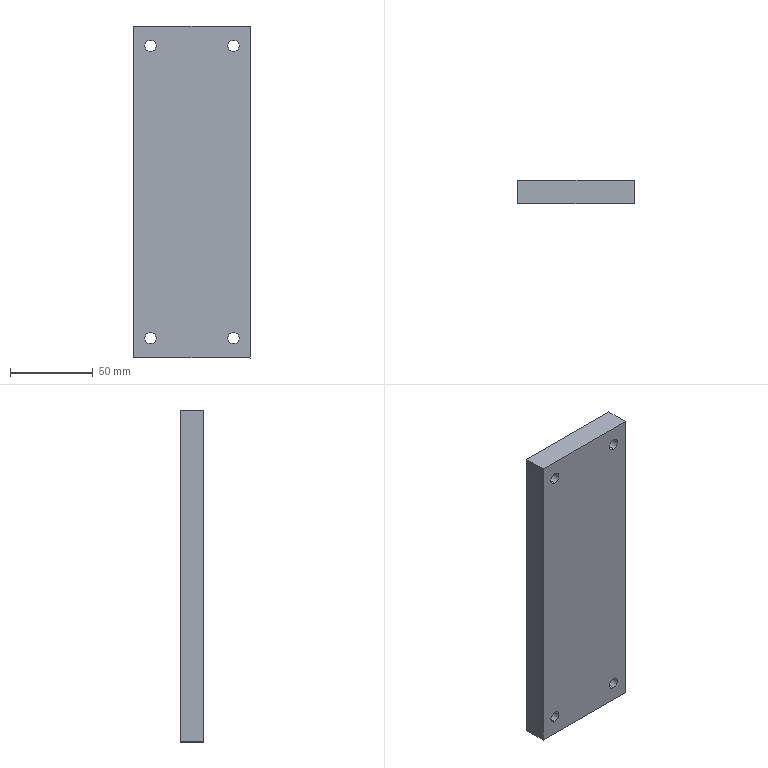Part | SolidWorks | features HoleWzd 2, Extrusion 1 | 1 solid | 14 faces | box 70 x 14 x 200 mm | volume 193966 mm3 | cylinder 8 | plane 6 | commonest cylinder face diameters 6.8 x8
STEP:
#1=CARTESIAN_POINT('',(60.,14.,-184.6));
#2=VERTEX_POINT('',#1);
#3=CARTESIAN_POINT('',(60.,14.,-191.4));
#4=VERTEX_POINT('',#3);
#5=CARTESIAN_POINT('',(60.,14.,-188.));
#6=DIRECTION('',(0.,-1.,0.));
#7=DIRECTION('',(0.,0.,-1.));
#8=AXIS2_PLACEMENT_3D('',#5,#6,#7);
#9=CIRCLE('',#8,3.4);
#10=EDGE_CURVE('',#2,#4,#9,.T.);
#11=ORIENTED_EDGE('',*,*,#10,.F.);
#12=CARTESIAN_POINT('',(60.,0.,-184.6));
#13=VERTEX_POINT('',#12);
#14=CARTESIAN_POINT('',(60.,0.,-184.6));
#15=DIRECTION('',(0.,-1.,0.));
#16=VECTOR('',#15,1000.);
#17=LINE('',#14,#16);
#18=EDGE_CURVE('',#2,#13,#17,.T.);
#19=ORIENTED_EDGE('',*,*,#18,.T.);
#20=CARTESIAN_POINT('',(60.,0.,-191.4));
#21=VERTEX_POINT('',#20);
#22=CARTESIAN_POINT('',(60.,0.,-188.));
#23=DIRECTION('',(0.,-1.,0.));
#24=DIRECTION('',(0.,0.,-1.));
#25=AXIS2_PLACEMENT_3D('',#22,#23,#24);
#26=CIRCLE('',#25,3.4);
#27=EDGE_CURVE('',#13,#21,#26,.T.);
#28=ORIENTED_EDGE('',*,*,#27,.T.);
#29=CARTESIAN_POINT('',(60.,0.,-191.4));
#30=DIRECTION('',(0.,-1.,0.));
#31=VECTOR('',#30,1000.);
#32=LINE('',#29,#31);
#33=EDGE_CURVE('',#4,#21,#32,.T.);
#34=ORIENTED_EDGE('',*,*,#33,.F.);
#35=EDGE_LOOP('',(#11,#19,#28,#34));
#36=FACE_OUTER_BOUND('',#35,.T.);
#37=CARTESIAN_POINT('',(60.,0.,-188.));
#38=DIRECTION('',(0.,-1.,0.));
#39=DIRECTION('',(0.,0.,-1.));
#40=AXIS2_PLACEMENT_3D('',#37,#38,#39);
#41=CYLINDRICAL_SURFACE('',#40,3.4);
#42=ADVANCED_FACE('',(#36),#41,.F.);
#43=CARTESIAN_POINT('',(10.,14.,-184.6));
#44=VERTEX_POINT('',#43);
#45=CARTESIAN_POINT('',(10.,14.,-191.4));
#46=VERTEX_POINT('',#45);
#47=CARTESIAN_POINT('',(10.,14.,-188.));
#48=DIRECTION('',(0.,-1.,0.));
#49=DIRECTION('',(0.,0.,-1.));
#50=AXIS2_PLACEMENT_3D('',#47,#48,#49);
#51=CIRCLE('',#50,3.4);
#52=EDGE_CURVE('',#44,#46,#51,.T.);
#53=ORIENTED_EDGE('',*,*,#52,.F.);
#54=CARTESIAN_POINT('',(10.,0.,-184.6));
#55=VERTEX_POINT('',#54);
#56=CARTESIAN_POINT('',(10.,0.,-184.6));
#57=DIRECTION('',(0.,-1.,0.));
#58=VECTOR('',#57,1000.);
#59=LINE('',#56,#58);
#60=EDGE_CURVE('',#44,#55,#59,.T.);
#61=ORIENTED_EDGE('',*,*,#60,.T.);
#62=CARTESIAN_POINT('',(10.,0.,-191.4));
#63=VERTEX_POINT('',#62);
#64=CARTESIAN_POINT('',(10.,0.,-188.));
#65=DIRECTION('',(0.,-1.,0.));
#66=DIRECTION('',(0.,0.,-1.));
#67=AXIS2_PLACEMENT_3D('',#64,#65,#66);
#68=CIRCLE('',#67,3.4);
#69=EDGE_CURVE('',#55,#63,#68,.T.);
#70=ORIENTED_EDGE('',*,*,#69,.T.);
#71=CARTESIAN_POINT('',(10.,0.,-191.4));
#72=DIRECTION('',(0.,-1.,0.));
#73=VECTOR('',#72,1000.);
#74=LINE('',#71,#73);
#75=EDGE_CURVE('',#46,#63,#74,.T.);
#76=ORIENTED_EDGE('',*,*,#75,.F.);
#77=EDGE_LOOP('',(#53,#61,#70,#76));
#78=FACE_OUTER_BOUND('',#77,.T.);
#79=CARTESIAN_POINT('',(10.,0.,-188.));
#80=DIRECTION('',(0.,-1.,0.));
#81=DIRECTION('',(0.,0.,-1.));
#82=AXIS2_PLACEMENT_3D('',#79,#80,#81);
#83=CYLINDRICAL_SURFACE('',#82,3.4);
#84=ADVANCED_FACE('',(#78),#83,.F.);
#85=CARTESIAN_POINT('',(10.,14.,-8.6));
#86=VERTEX_POINT('',#85);
#87=CARTESIAN_POINT('',(10.,14.,-15.4));
#88=VERTEX_POINT('',#87);
#89=CARTESIAN_POINT('',(10.,14.,-12.));
#90=DIRECTION('',(0.,-1.,0.));
#91=DIRECTION('',(0.,0.,-1.));
#92=AXIS2_PLACEMENT_3D('',#89,#90,#91);
#93=CIRCLE('',#92,3.4);
#94=EDGE_CURVE('',#86,#88,#93,.T.);
#95=ORIENTED_EDGE('',*,*,#94,.F.);
#96=CARTESIAN_POINT('',(10.,0.,-8.6));
#97=VERTEX_POINT('',#96);
#98=CARTESIAN_POINT('',(10.,0.,-8.6));
#99=DIRECTION('',(0.,-1.,0.));
#100=VECTOR('',#99,1000.);
#101=LINE('',#98,#100);
#102=EDGE_CURVE('',#86,#97,#101,.T.);
#103=ORIENTED_EDGE('',*,*,#102,.T.);
#104=CARTESIAN_POINT('',(10.,0.,-15.4));
#105=VERTEX_POINT('',#104);
#106=CARTESIAN_POINT('',(10.,0.,-12.));
#107=DIRECTION('',(0.,-1.,0.));
#108=DIRECTION('',(0.,0.,-1.));
#109=AXIS2_PLACEMENT_3D('',#106,#107,#108);
#110=CIRCLE('',#109,3.4);
#111=EDGE_CURVE('',#97,#105,#110,.T.);
#112=ORIENTED_EDGE('',*,*,#111,.T.);
#113=CARTESIAN_POINT('',(10.,0.,-15.4));
#114=DIRECTION('',(0.,-1.,0.));
#115=VECTOR('',#114,1000.);
#116=LINE('',#113,#115);
#117=EDGE_CURVE('',#88,#105,#116,.T.);
#118=ORIENTED_EDGE('',*,*,#117,.F.);
#119=EDGE_LOOP('',(#95,#103,#112,#118));
#120=FACE_OUTER_BOUND('',#119,.T.);
#121=CARTESIAN_POINT('',(10.,0.,-12.));
#122=DIRECTION('',(0.,-1.,0.));
#123=DIRECTION('',(0.,0.,-1.));
#124=AXIS2_PLACEMENT_3D('',#121,#122,#123);
#125=CYLINDRICAL_SURFACE('',#124,3.4);
#126=ADVANCED_FACE('',(#120),#125,.F.);
#127=CARTESIAN_POINT('',(60.,14.,-8.6));
#128=VERTEX_POINT('',#127);
#129=CARTESIAN_POINT('',(60.,14.,-15.4));
#130=VERTEX_POINT('',#129);
#131=CARTESIAN_POINT('',(60.,14.,-12.));
#132=DIRECTION('',(0.,-1.,0.));
#133=DIRECTION('',(0.,0.,-1.));
#134=AXIS2_PLACEMENT_3D('',#131,#132,#133);
#135=CIRCLE('',#134,3.4);
#136=EDGE_CURVE('',#128,#130,#135,.T.);
#137=ORIENTED_EDGE('',*,*,#136,.F.);
#138=CARTESIAN_POINT('',(60.,0.,-8.6));
#139=VERTEX_POINT('',#138);
#140=CARTESIAN_POINT('',(60.,0.,-8.6));
#141=DIRECTION('',(0.,-1.,0.));
#142=VECTOR('',#141,1000.);
#143=LINE('',#140,#142);
#144=EDGE_CURVE('',#128,#139,#143,.T.);
#145=ORIENTED_EDGE('',*,*,#144,.T.);
#146=CARTESIAN_POINT('',(60.,0.,-15.4));
#147=VERTEX_POINT('',#146);
#148=CARTESIAN_POINT('',(60.,0.,-12.));
#149=DIRECTION('',(0.,-1.,0.));
#150=DIRECTION('',(0.,0.,-1.));
#151=AXIS2_PLACEMENT_3D('',#148,#149,#150);
#152=CIRCLE('',#151,3.4);
#153=EDGE_CURVE('',#139,#147,#152,.T.);
#154=ORIENTED_EDGE('',*,*,#153,.T.);
#155=CARTESIAN_POINT('',(60.,0.,-15.4));
#156=DIRECTION('',(0.,-1.,0.));
#157=VECTOR('',#156,1000.);
#158=LINE('',#155,#157);
#159=EDGE_CURVE('',#130,#147,#158,.T.);
#160=ORIENTED_EDGE('',*,*,#159,.F.);
#161=EDGE_LOOP('',(#137,#145,#154,#160));
#162=FACE_OUTER_BOUND('',#161,.T.);
#163=CARTESIAN_POINT('',(60.,0.,-12.));
#164=DIRECTION('',(0.,-1.,0.));
#165=DIRECTION('',(0.,0.,-1.));
#166=AXIS2_PLACEMENT_3D('',#163,#164,#165);
#167=CYLINDRICAL_SURFACE('',#166,3.4);
#168=ADVANCED_FACE('',(#162),#167,.F.);
#169=CARTESIAN_POINT('',(70.,0.,0.));
#170=VERTEX_POINT('',#169);
#171=CARTESIAN_POINT('',(70.,0.,-200.));
#172=VERTEX_POINT('',#171);
#173=CARTESIAN_POINT('',(70.,0.,0.));
#174=DIRECTION('',(0.,0.,-1.));
#175=VECTOR('',#174,1000.);
#176=LINE('',#173,#175);
#177=EDGE_CURVE('',#170,#172,#176,.T.);
#178=ORIENTED_EDGE('',*,*,#177,.T.);
#179=CARTESIAN_POINT('',(70.,14.,-200.));
#180=VERTEX_POINT('',#179);
#181=CARTESIAN_POINT('',(70.,14.,-200.));
#182=DIRECTION('',(0.,-1.,0.));
#183=VECTOR('',#182,1000.);
#184=LINE('',#181,#183);
#185=EDGE_CURVE('',#180,#172,#184,.T.);
#186=ORIENTED_EDGE('',*,*,#185,.F.);
#187=CARTESIAN_POINT('',(70.,14.,0.));
#188=VERTEX_POINT('',#187);
#189=CARTESIAN_POINT('',(70.,14.,0.));
#190=DIRECTION('',(0.,0.,-1.));
#191=VECTOR('',#190,1000.);
#192=LINE('',#189,#191);
#193=EDGE_CURVE('',#188,#180,#192,.T.);
#194=ORIENTED_EDGE('',*,*,#193,.F.);
#195=CARTESIAN_POINT('',(70.,14.,0.));
#196=DIRECTION('',(0.,-1.,0.));
#197=VECTOR('',#196,1000.);
#198=LINE('',#195,#197);
#199=EDGE_CURVE('',#188,#170,#198,.T.);
#200=ORIENTED_EDGE('',*,*,#199,.T.);
#201=EDGE_LOOP('',(#178,#186,#194,#200));
#202=FACE_OUTER_BOUND('',#201,.T.);
#203=CARTESIAN_POINT('',(70.,14.,0.));
#204=DIRECTION('',(-1.,0.,0.));
#205=DIRECTION('',(0.,0.,1.));
#206=AXIS2_PLACEMENT_3D('',#203,#204,#205);
#207=PLANE('',#206);
#208=ADVANCED_FACE('',(#202),#207,.F.);
#209=CARTESIAN_POINT('',(0.,0.,-200.));
#210=VERTEX_POINT('',#209);
#211=CARTESIAN_POINT('',(0.,0.,-200.));
#212=DIRECTION('',(-1.,0.,0.));
#213=VECTOR('',#212,1000.);
#214=LINE('',#211,#213);
#215=EDGE_CURVE('',#172,#210,#214,.T.);
#216=ORIENTED_EDGE('',*,*,#215,.T.);
#217=CARTESIAN_POINT('',(0.,14.,-200.));
#218=VERTEX_POINT('',#217);
#219=CARTESIAN_POINT('',(0.,14.,-200.));
#220=DIRECTION('',(0.,-1.,0.));
#221=VECTOR('',#220,1000.);
#222=LINE('',#219,#221);
#223=EDGE_CURVE('',#218,#210,#222,.T.);
#224=ORIENTED_EDGE('',*,*,#223,.F.);
#225=CARTESIAN_POINT('',(0.,14.,-200.));
#226=DIRECTION('',(-1.,0.,0.));
#227=VECTOR('',#226,1000.);
#228=LINE('',#225,#227);
#229=EDGE_CURVE('',#180,#218,#228,.T.);
#230=ORIENTED_EDGE('',*,*,#229,.F.);
#231=ORIENTED_EDGE('',*,*,#185,.T.);
#232=EDGE_LOOP('',(#216,#224,#230,#231));
#233=FACE_OUTER_BOUND('',#232,.T.);
#234=CARTESIAN_POINT('',(0.,14.,-200.));
#235=DIRECTION('',(0.,0.,1.));
#236=DIRECTION('',(1.,0.,0.));
#237=AXIS2_PLACEMENT_3D('',#234,#235,#236);
#238=PLANE('',#237);
#239=ADVANCED_FACE('',(#233),#238,.F.);
#240=CARTESIAN_POINT('',(0.,0.,0.));
#241=VERTEX_POINT('',#240);
#242=CARTESIAN_POINT('',(0.,0.,0.));
#243=DIRECTION('',(0.,0.,1.));
#244=VECTOR('',#243,1000.);
#245=LINE('',#242,#244);
#246=EDGE_CURVE('',#210,#241,#245,.T.);
#247=ORIENTED_EDGE('',*,*,#246,.T.);
#248=CARTESIAN_POINT('',(0.,14.,0.));
#249=VERTEX_POINT('',#248);
#250=CARTESIAN_POINT('',(0.,14.,0.));
#251=DIRECTION('',(0.,-1.,0.));
#252=VECTOR('',#251,1000.);
#253=LINE('',#250,#252);
#254=EDGE_CURVE('',#249,#241,#253,.T.);
#255=ORIENTED_EDGE('',*,*,#254,.F.);
#256=CARTESIAN_POINT('',(0.,14.,0.));
#257=DIRECTION('',(0.,0.,1.));
#258=VECTOR('',#257,1000.);
#259=LINE('',#256,#258);
#260=EDGE_CURVE('',#218,#249,#259,.T.);
#261=ORIENTED_EDGE('',*,*,#260,.F.);
#262=ORIENTED_EDGE('',*,*,#223,.T.);
#263=EDGE_LOOP('',(#247,#255,#261,#262));
#264=FACE_OUTER_BOUND('',#263,.T.);
#265=CARTESIAN_POINT('',(0.,14.,0.));
#266=DIRECTION('',(1.,0.,0.));
#267=DIRECTION('',(0.,0.,-1.));
#268=AXIS2_PLACEMENT_3D('',#265,#266,#267);
#269=PLANE('',#268);
#270=ADVANCED_FACE('',(#264),#269,.F.);
#271=CARTESIAN_POINT('',(0.,0.,0.));
#272=DIRECTION('',(1.,0.,0.));
#273=VECTOR('',#272,1000.);
#274=LINE('',#271,#273);
#275=EDGE_CURVE('',#241,#170,#274,.T.);
#276=ORIENTED_EDGE('',*,*,#275,.T.);
#277=ORIENTED_EDGE('',*,*,#199,.F.);
#278=CARTESIAN_POINT('',(0.,14.,0.));
#279=DIRECTION('',(1.,0.,0.));
#280=VECTOR('',#279,1000.);
#281=LINE('',#278,#280);
#282=EDGE_CURVE('',#249,#188,#281,.T.);
#283=ORIENTED_EDGE('',*,*,#282,.F.);
#284=ORIENTED_EDGE('',*,*,#254,.T.);
#285=EDGE_LOOP('',(#276,#277,#283,#284));
#286=FACE_OUTER_BOUND('',#285,.T.);
#287=CARTESIAN_POINT('',(0.,14.,0.));
#288=DIRECTION('',(0.,0.,-1.));
#289=DIRECTION('',(-1.,0.,0.));
#290=AXIS2_PLACEMENT_3D('',#287,#288,#289);
#291=PLANE('',#290);
#292=ADVANCED_FACE('',(#286),#291,.F.);
#293=CARTESIAN_POINT('',(60.,14.,-188.));
#294=DIRECTION('',(0.,-1.,0.));
#295=DIRECTION('',(0.,0.,-1.));
#296=AXIS2_PLACEMENT_3D('',#293,#294,#295);
#297=CIRCLE('',#296,3.4);
#298=EDGE_CURVE('',#4,#2,#297,.T.);
#299=ORIENTED_EDGE('',*,*,#298,.T.);
#300=ORIENTED_EDGE('',*,*,#10,.T.);
#301=EDGE_LOOP('',(#299,#300));
#302=FACE_BOUND('',#301,.T.);
#303=CARTESIAN_POINT('',(10.,14.,-188.));
#304=DIRECTION('',(0.,-1.,0.));
#305=DIRECTION('',(0.,0.,-1.));
#306=AXIS2_PLACEMENT_3D('',#303,#304,#305);
#307=CIRCLE('',#306,3.4);
#308=EDGE_CURVE('',#46,#44,#307,.T.);
#309=ORIENTED_EDGE('',*,*,#308,.T.);
#310=ORIENTED_EDGE('',*,*,#52,.T.);
#311=EDGE_LOOP('',(#309,#310));
#312=FACE_BOUND('',#311,.T.);
#313=CARTESIAN_POINT('',(10.,14.,-12.));
#314=DIRECTION('',(0.,-1.,0.));
#315=DIRECTION('',(0.,0.,-1.));
#316=AXIS2_PLACEMENT_3D('',#313,#314,#315);
#317=CIRCLE('',#316,3.4);
#318=EDGE_CURVE('',#88,#86,#317,.T.);
#319=ORIENTED_EDGE('',*,*,#318,.T.);
#320=ORIENTED_EDGE('',*,*,#94,.T.);
#321=EDGE_LOOP('',(#319,#320));
#322=FACE_BOUND('',#321,.T.);
#323=CARTESIAN_POINT('',(60.,14.,-12.));
#324=DIRECTION('',(0.,-1.,0.));
#325=DIRECTION('',(0.,0.,-1.));
#326=AXIS2_PLACEMENT_3D('',#323,#324,#325);
#327=CIRCLE('',#326,3.4);
#328=EDGE_CURVE('',#130,#128,#327,.T.);
#329=ORIENTED_EDGE('',*,*,#328,.T.);
#330=ORIENTED_EDGE('',*,*,#136,.T.);
#331=EDGE_LOOP('',(#329,#330));
#332=FACE_BOUND('',#331,.T.);
#333=ORIENTED_EDGE('',*,*,#193,.T.);
#334=ORIENTED_EDGE('',*,*,#229,.T.);
#335=ORIENTED_EDGE('',*,*,#260,.T.);
#336=ORIENTED_EDGE('',*,*,#282,.T.);
#337=EDGE_LOOP('',(#333,#334,#335,#336));
#338=FACE_OUTER_BOUND('',#337,.T.);
#339=CARTESIAN_POINT('',(0.,14.,0.));
#340=DIRECTION('',(0.,-1.,0.));
#341=DIRECTION('',(0.,0.,-1.));
#342=AXIS2_PLACEMENT_3D('',#339,#340,#341);
#343=PLANE('',#342);
#344=ADVANCED_FACE('',(#302,#312,#322,#332,#338),#343,.F.);
#345=CARTESIAN_POINT('',(60.,0.,-188.));
#346=DIRECTION('',(0.,-1.,0.));
#347=DIRECTION('',(0.,0.,-1.));
#348=AXIS2_PLACEMENT_3D('',#345,#346,#347);
#349=CIRCLE('',#348,3.4);
#350=EDGE_CURVE('',#21,#13,#349,.T.);
#351=ORIENTED_EDGE('',*,*,#350,.F.);
#352=ORIENTED_EDGE('',*,*,#27,.F.);
#353=EDGE_LOOP('',(#351,#352));
#354=FACE_BOUND('',#353,.T.);
#355=CARTESIAN_POINT('',(10.,0.,-188.));
#356=DIRECTION('',(0.,-1.,0.));
#357=DIRECTION('',(0.,0.,-1.));
#358=AXIS2_PLACEMENT_3D('',#355,#356,#357);
#359=CIRCLE('',#358,3.4);
#360=EDGE_CURVE('',#63,#55,#359,.T.);
#361=ORIENTED_EDGE('',*,*,#360,.F.);
#362=ORIENTED_EDGE('',*,*,#69,.F.);
#363=EDGE_LOOP('',(#361,#362));
#364=FACE_BOUND('',#363,.T.);
#365=CARTESIAN_POINT('',(10.,0.,-12.));
#366=DIRECTION('',(0.,-1.,0.));
#367=DIRECTION('',(0.,0.,-1.));
#368=AXIS2_PLACEMENT_3D('',#365,#366,#367);
#369=CIRCLE('',#368,3.4);
#370=EDGE_CURVE('',#105,#97,#369,.T.);
#371=ORIENTED_EDGE('',*,*,#370,.F.);
#372=ORIENTED_EDGE('',*,*,#111,.F.);
#373=EDGE_LOOP('',(#371,#372));
#374=FACE_BOUND('',#373,.T.);
#375=CARTESIAN_POINT('',(60.,0.,-12.));
#376=DIRECTION('',(0.,-1.,0.));
#377=DIRECTION('',(0.,0.,-1.));
#378=AXIS2_PLACEMENT_3D('',#375,#376,#377);
#379=CIRCLE('',#378,3.4);
#380=EDGE_CURVE('',#147,#139,#379,.T.);
#381=ORIENTED_EDGE('',*,*,#380,.F.);
#382=ORIENTED_EDGE('',*,*,#153,.F.);
#383=EDGE_LOOP('',(#381,#382));
#384=FACE_BOUND('',#383,.T.);
#385=ORIENTED_EDGE('',*,*,#177,.F.);
#386=ORIENTED_EDGE('',*,*,#275,.F.);
#387=ORIENTED_EDGE('',*,*,#246,.F.);
#388=ORIENTED_EDGE('',*,*,#215,.F.);
#389=EDGE_LOOP('',(#385,#386,#387,#388));
#390=FACE_OUTER_BOUND('',#389,.T.);
#391=CARTESIAN_POINT('',(0.,0.,0.));
#392=DIRECTION('',(0.,-1.,0.));
#393=DIRECTION('',(0.,0.,-1.));
#394=AXIS2_PLACEMENT_3D('',#391,#392,#393);
#395=PLANE('',#394);
#396=ADVANCED_FACE('',(#354,#364,#374,#384,#390),#395,.T.);
#397=ORIENTED_EDGE('',*,*,#144,.F.);
#398=ORIENTED_EDGE('',*,*,#328,.F.);
#399=ORIENTED_EDGE('',*,*,#159,.T.);
#400=ORIENTED_EDGE('',*,*,#380,.T.);
#401=EDGE_LOOP('',(#397,#398,#399,#400));
#402=FACE_OUTER_BOUND('',#401,.T.);
#403=CARTESIAN_POINT('',(60.,0.,-12.));
#404=DIRECTION('',(0.,-1.,0.));
#405=DIRECTION('',(0.,0.,-1.));
#406=AXIS2_PLACEMENT_3D('',#403,#404,#405);
#407=CYLINDRICAL_SURFACE('',#406,3.4);
#408=ADVANCED_FACE('',(#402),#407,.F.);
#409=ORIENTED_EDGE('',*,*,#102,.F.);
#410=ORIENTED_EDGE('',*,*,#318,.F.);
#411=ORIENTED_EDGE('',*,*,#117,.T.);
#412=ORIENTED_EDGE('',*,*,#370,.T.);
#413=EDGE_LOOP('',(#409,#410,#411,#412));
#414=FACE_OUTER_BOUND('',#413,.T.);
#415=CARTESIAN_POINT('',(10.,0.,-12.));
#416=DIRECTION('',(0.,-1.,0.));
#417=DIRECTION('',(0.,0.,-1.));
#418=AXIS2_PLACEMENT_3D('',#415,#416,#417);
#419=CYLINDRICAL_SURFACE('',#418,3.4);
#420=ADVANCED_FACE('',(#414),#419,.F.);
#421=ORIENTED_EDGE('',*,*,#60,.F.);
#422=ORIENTED_EDGE('',*,*,#308,.F.);
#423=ORIENTED_EDGE('',*,*,#75,.T.);
#424=ORIENTED_EDGE('',*,*,#360,.T.);
#425=EDGE_LOOP('',(#421,#422,#423,#424));
#426=FACE_OUTER_BOUND('',#425,.T.);
#427=CARTESIAN_POINT('',(10.,0.,-188.));
#428=DIRECTION('',(0.,-1.,0.));
#429=DIRECTION('',(0.,0.,-1.));
#430=AXIS2_PLACEMENT_3D('',#427,#428,#429);
#431=CYLINDRICAL_SURFACE('',#430,3.4);
#432=ADVANCED_FACE('',(#426),#431,.F.);
#433=ORIENTED_EDGE('',*,*,#18,.F.);
#434=ORIENTED_EDGE('',*,*,#298,.F.);
#435=ORIENTED_EDGE('',*,*,#33,.T.);
#436=ORIENTED_EDGE('',*,*,#350,.T.);
#437=EDGE_LOOP('',(#433,#434,#435,#436));
#438=FACE_OUTER_BOUND('',#437,.T.);
#439=CARTESIAN_POINT('',(60.,0.,-188.));
#440=DIRECTION('',(0.,-1.,0.));
#441=DIRECTION('',(0.,0.,-1.));
#442=AXIS2_PLACEMENT_3D('',#439,#440,#441);
#443=CYLINDRICAL_SURFACE('',#442,3.4);
#444=ADVANCED_FACE('',(#438),#443,.F.);
#445=CLOSED_SHELL('',(#42,#84,#126,#168,#208,#239,#270,#292,#344,#396,#408,#420,#432,#444));
#446=MANIFOLD_SOLID_BREP('',#445);
#447=CARTESIAN_POINT('',(0.,0.,0.));
#448=DIRECTION('',(0.,0.,1.));
#449=DIRECTION('',(1.,0.,0.));
#450=AXIS2_PLACEMENT_3D('',#447,#448,#449);
#451=(LENGTH_UNIT()NAMED_UNIT(*)SI_UNIT(.MILLI.,.METRE.));
#452=UNCERTAINTY_MEASURE_WITH_UNIT(LENGTH_MEASURE(0.00001),#451,'','');
#453=(NAMED_UNIT(*)PLANE_ANGLE_UNIT()SI_UNIT($,.RADIAN.));
#454=(NAMED_UNIT(*)SI_UNIT($,.STERADIAN.)SOLID_ANGLE_UNIT());
#455=(GEOMETRIC_REPRESENTATION_CONTEXT(3)GLOBAL_UNCERTAINTY_ASSIGNED_CONTEXT((#452))GLOBAL_UNIT_ASSIGNED_CONTEXT((#451,#453,#454))REPRESENTATION_CONTEXT('',''));
#456=ADVANCED_BREP_SHAPE_REPRESENTATION('',(#446,#450),#455);